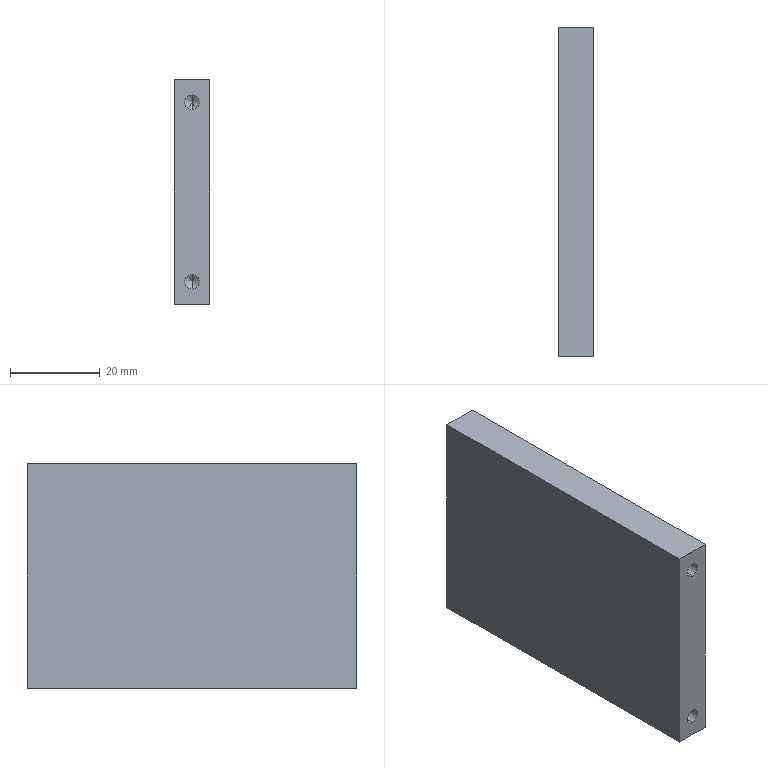Part | STEP file | 0243_203_Plate | 1 solid | 22 faces | box 8 x 73.5 x 50 mm | volume 28975 mm3 | cylinder 8 | cone 8 | plane 6 | commonest cylinder face diameters 3.3 x8